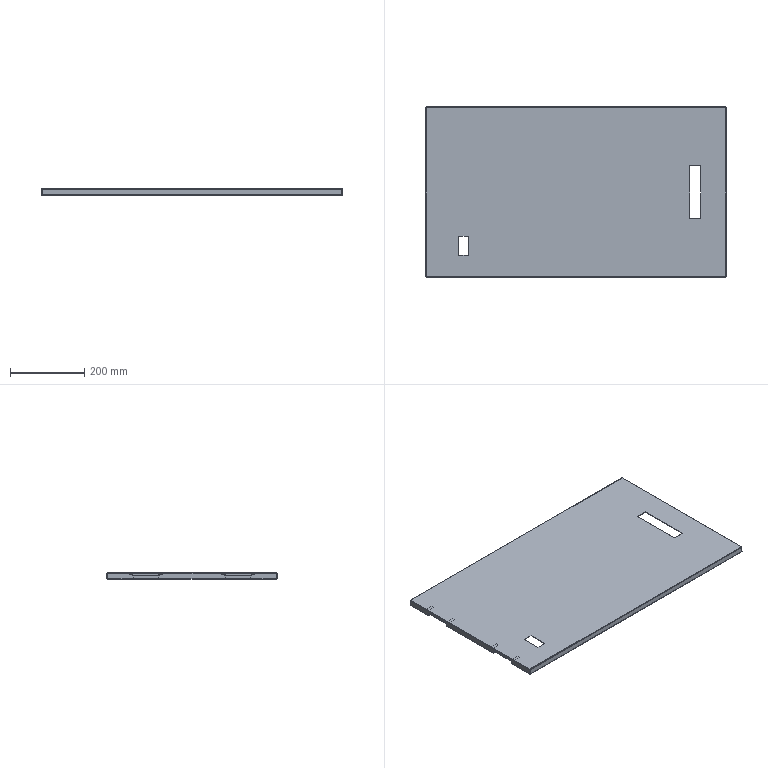Part | NX | features BREP 3 | 3 solids | 182 faces | box 810 x 458 x 16.5 mm | volume 636451 mm3 | plane 118 | cylinder 48 | spline 16 | commonest cylinder face diameters 0.02 x18 3.02 x18 3.2 x12